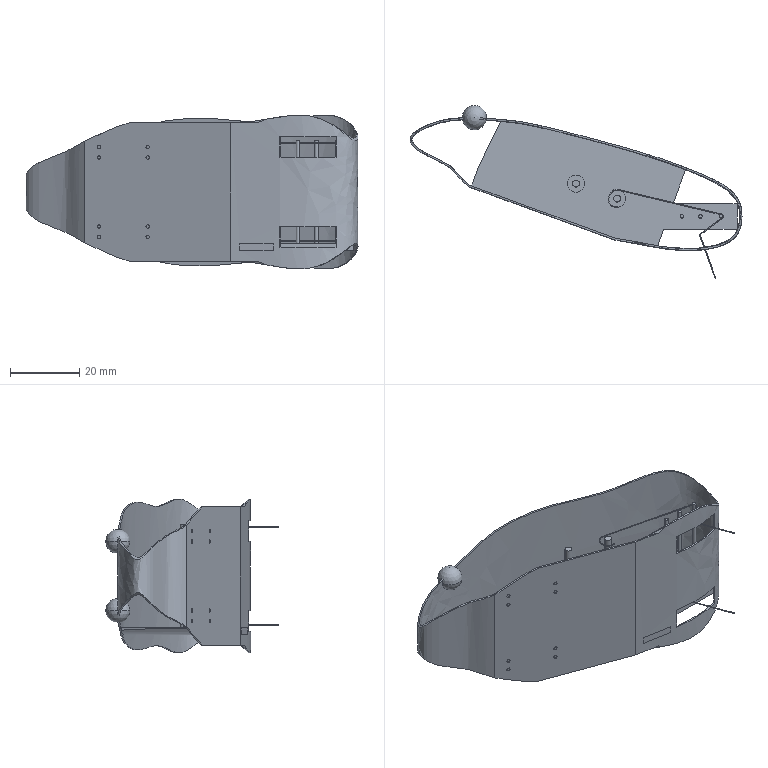Part | SolidWorks | features ICE 13, MirrorPattern 3, Extrusion 1, Fillet 1, Revolution 1, Sweep 1 | 1 solid | 111 faces | box 96.052 x 49.979 x 44.528 mm | volume 8210 mm3 | cylinder 43 | plane 42 | spline 14 | torus 6 | sphere 6 | commonest cylinder face diameters 1 x22 0.2 x12 2 x4 5 x4 40 x1